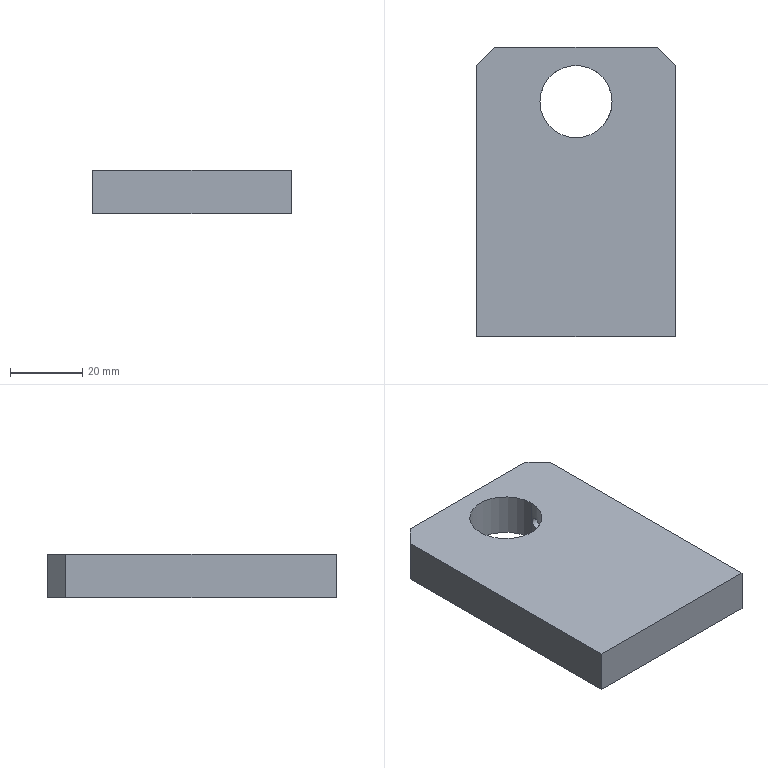Part | SolidWorks | features ICE 3, 3DProfileFeature 1, Chamfer 1, Extrusion 1, HoleWzd 1 | 1 solid | 12 faces | box 55 x 80 x 12 mm | volume 48578 mm3 | plane 8 | cylinder 4 | commonest cylinder face diameters 3.3 x2 20 x2
STEP:
#1=CARTESIAN_POINT('',(9.798,23.,7.65));
#2=VERTEX_POINT('',#1);
#3=CARTESIAN_POINT('',(9.798,23.,4.35));
#4=VERTEX_POINT('',#3);
#5=CARTESIAN_POINT('',(9.798,23.,7.65));
#6=CARTESIAN_POINT('',(9.754,22.785,7.65));
#7=CARTESIAN_POINT('',(9.702,22.57,7.607));
#8=CARTESIAN_POINT('',(9.595,22.176,7.445));
#9=CARTESIAN_POINT('',(9.539,21.994,7.325));
#10=CARTESIAN_POINT('',(9.463,21.766,7.1));
#11=CARTESIAN_POINT('',(9.439,21.696,7.016));
#12=CARTESIAN_POINT('',(9.395,21.575,6.838));
#13=CARTESIAN_POINT('',(9.376,21.523,6.744));
#14=CARTESIAN_POINT('',(9.344,21.438,6.543));
#15=CARTESIAN_POINT('',(9.332,21.405,6.437));
#16=CARTESIAN_POINT('',(9.315,21.361,6.223));
#17=CARTESIAN_POINT('',(9.31,21.35,6.114));
#18=CARTESIAN_POINT('',(9.31,21.35,5.891));
#19=CARTESIAN_POINT('',(9.314,21.361,5.782));
#20=CARTESIAN_POINT('',(9.331,21.404,5.567));
#21=CARTESIAN_POINT('',(9.344,21.437,5.461));
#22=CARTESIAN_POINT('',(9.391,21.564,5.159));
#23=CARTESIAN_POINT('',(9.437,21.688,4.977));
#24=CARTESIAN_POINT('',(9.538,21.992,4.676));
#25=CARTESIAN_POINT('',(9.595,22.174,4.556));
#26=CARTESIAN_POINT('',(9.675,22.469,4.434));
#27=CARTESIAN_POINT('',(9.702,22.573,4.403));
#28=CARTESIAN_POINT('',(9.752,22.784,4.361));
#29=CARTESIAN_POINT('',(9.776,22.891,4.35));
#30=CARTESIAN_POINT('',(9.798,23.,4.35));
#31=B_SPLINE_CURVE_WITH_KNOTS('',3,(#5,#6,#7,#8,#9,#10,#11,#12,#13,#14,#15,#16,#17,#18,#19,#20,#21,#22,#23,#24,#25,#26,#27,#28,#29,#30),.UNSPECIFIED.,.F.,.F.,(4,2,2,2,2,2,2,2,2,2,2,2,4),(0.005184,0.005841,0.006499,0.006828,0.007157,0.007485,0.007814,0.008143,0.008472,0.00913,0.009787,0.01012,0.01044),.UNSPECIFIED.);
#32=EDGE_CURVE('',#2,#4,#31,.T.);
#33=ORIENTED_EDGE('',*,*,#32,.F.);
#34=CARTESIAN_POINT('',(27.5,23.,7.65));
#35=VERTEX_POINT('',#34);
#36=CARTESIAN_POINT('',(27.5,23.,7.65));
#37=DIRECTION('',(1.,0.,0.));
#38=VECTOR('',#37,1000.);
#39=LINE('',#36,#38);
#40=EDGE_CURVE('',#2,#35,#39,.T.);
#41=ORIENTED_EDGE('',*,*,#40,.T.);
#42=CARTESIAN_POINT('',(27.5,23.,4.35));
#43=VERTEX_POINT('',#42);
#44=CARTESIAN_POINT('',(27.5,23.,6.));
#45=DIRECTION('',(1.,0.,0.));
#46=DIRECTION('',(0.,0.,-1.));
#47=AXIS2_PLACEMENT_3D('',#44,#45,#46);
#48=CIRCLE('',#47,1.65);
#49=EDGE_CURVE('',#35,#43,#48,.T.);
#50=ORIENTED_EDGE('',*,*,#49,.T.);
#51=CARTESIAN_POINT('',(27.5,23.,4.35));
#52=DIRECTION('',(1.,0.,0.));
#53=VECTOR('',#52,1000.);
#54=LINE('',#51,#53);
#55=EDGE_CURVE('',#4,#43,#54,.T.);
#56=ORIENTED_EDGE('',*,*,#55,.F.);
#57=EDGE_LOOP('',(#33,#41,#50,#56));
#58=FACE_OUTER_BOUND('',#57,.T.);
#59=CARTESIAN_POINT('',(27.5,23.,6.));
#60=DIRECTION('',(1.,0.,0.));
#61=DIRECTION('',(0.,0.,-1.));
#62=AXIS2_PLACEMENT_3D('',#59,#60,#61);
#63=CYLINDRICAL_SURFACE('',#62,1.65);
#64=ADVANCED_FACE('',(#58),#63,.F.);
#65=CARTESIAN_POINT('',(9.798,23.,4.35));
#66=CARTESIAN_POINT('',(9.82,23.107,4.35));
#67=CARTESIAN_POINT('',(9.84,23.213,4.36));
#68=CARTESIAN_POINT('',(9.875,23.422,4.401));
#69=CARTESIAN_POINT('',(9.891,23.527,4.433));
#70=CARTESIAN_POINT('',(9.919,23.726,4.514));
#71=CARTESIAN_POINT('',(9.931,23.821,4.565));
#72=CARTESIAN_POINT('',(9.95,24.001,4.684));
#73=CARTESIAN_POINT('',(9.958,24.086,4.753));
#74=CARTESIAN_POINT('',(9.978,24.316,4.982));
#75=CARTESIAN_POINT('',(9.985,24.44,5.166));
#76=CARTESIAN_POINT('',(9.993,24.606,5.565));
#77=CARTESIAN_POINT('',(9.994,24.65,5.783));
#78=CARTESIAN_POINT('',(9.994,24.65,6.108));
#79=CARTESIAN_POINT('',(9.994,24.639,6.217));
#80=CARTESIAN_POINT('',(9.992,24.597,6.43));
#81=CARTESIAN_POINT('',(9.991,24.565,6.533));
#82=CARTESIAN_POINT('',(9.987,24.482,6.734));
#83=CARTESIAN_POINT('',(9.984,24.43,6.831));
#84=CARTESIAN_POINT('',(9.976,24.309,7.01));
#85=CARTESIAN_POINT('',(9.971,24.24,7.094));
#86=CARTESIAN_POINT('',(9.958,24.085,7.248));
#87=CARTESIAN_POINT('',(9.95,24.002,7.316));
#88=CARTESIAN_POINT('',(9.931,23.822,7.435));
#89=CARTESIAN_POINT('',(9.919,23.725,7.486));
#90=CARTESIAN_POINT('',(9.891,23.526,7.568));
#91=CARTESIAN_POINT('',(9.876,23.424,7.598));
#92=CARTESIAN_POINT('',(9.84,23.214,7.64));
#93=CARTESIAN_POINT('',(9.82,23.106,7.65));
#94=CARTESIAN_POINT('',(9.798,23.,7.65));
#95=B_SPLINE_CURVE_WITH_KNOTS('',3,(#65,#66,#67,#68,#69,#70,#71,#72,#73,#74,#75,#76,#77,#78,#79,#80,#81,#82,#83,#84,#85,#86,#87,#88,#89,#90,#91,#92,#93,#94),.UNSPECIFIED.,.F.,.F.,(4,2,2,2,2,2,2,2,2,2,2,2,2,2,4),(0.,0.000324,0.0006479,0.0009719,0.001296,0.001944,0.002592,0.002916,0.00324,0.003564,0.003888,0.004212,0.004536,0.00486,0.005184),.UNSPECIFIED.);
#96=EDGE_CURVE('',#4,#2,#95,.T.);
#97=ORIENTED_EDGE('',*,*,#96,.T.);
#98=ORIENTED_EDGE('',*,*,#32,.T.);
#99=EDGE_LOOP('',(#97,#98));
#100=FACE_BOUND('',#99,.T.);
#101=CARTESIAN_POINT('',(-10.,25.,12.));
#102=VERTEX_POINT('',#101);
#103=CARTESIAN_POINT('',(10.,25.,12.));
#104=VERTEX_POINT('',#103);
#105=CARTESIAN_POINT('',(0.,25.,12.));
#106=DIRECTION('',(0.,0.,1.));
#107=DIRECTION('',(-1.,0.,0.));
#108=AXIS2_PLACEMENT_3D('',#105,#106,#107);
#109=CIRCLE('',#108,10.);
#110=EDGE_CURVE('',#102,#104,#109,.T.);
#111=ORIENTED_EDGE('',*,*,#110,.T.);
#112=CARTESIAN_POINT('',(10.,25.,0.));
#113=VERTEX_POINT('',#112);
#114=CARTESIAN_POINT('',(10.,25.,12.001));
#115=DIRECTION('',(0.,0.,-1.));
#116=VECTOR('',#115,1000.);
#117=LINE('',#114,#116);
#118=EDGE_CURVE('',#104,#113,#117,.T.);
#119=ORIENTED_EDGE('',*,*,#118,.T.);
#120=CARTESIAN_POINT('',(-10.,25.,0.));
#121=VERTEX_POINT('',#120);
#122=CARTESIAN_POINT('',(0.,25.,0.));
#123=DIRECTION('',(0.,0.,-1.));
#124=DIRECTION('',(-1.,0.,0.));
#125=AXIS2_PLACEMENT_3D('',#122,#123,#124);
#126=CIRCLE('',#125,10.);
#127=EDGE_CURVE('',#113,#121,#126,.T.);
#128=ORIENTED_EDGE('',*,*,#127,.T.);
#129=CARTESIAN_POINT('',(-10.,25.,12.001));
#130=DIRECTION('',(0.,0.,-1.));
#131=VECTOR('',#130,1000.);
#132=LINE('',#129,#131);
#133=EDGE_CURVE('',#102,#121,#132,.T.);
#134=ORIENTED_EDGE('',*,*,#133,.F.);
#135=EDGE_LOOP('',(#111,#119,#128,#134));
#136=FACE_OUTER_BOUND('',#135,.T.);
#137=CARTESIAN_POINT('',(0.,25.,12.001));
#138=DIRECTION('',(0.,0.,-1.));
#139=DIRECTION('',(-1.,0.,0.));
#140=AXIS2_PLACEMENT_3D('',#137,#138,#139);
#141=CYLINDRICAL_SURFACE('',#140,10.);
#142=ADVANCED_FACE('',(#100,#136),#141,.F.);
#143=CARTESIAN_POINT('',(27.5,-40.,0.));
#144=VERTEX_POINT('',#143);
#145=CARTESIAN_POINT('',(27.5,35.,0.));
#146=VERTEX_POINT('',#145);
#147=CARTESIAN_POINT('',(27.5,-40.,0.));
#148=DIRECTION('',(0.,1.,0.));
#149=VECTOR('',#148,1000.);
#150=LINE('',#147,#149);
#151=EDGE_CURVE('',#144,#146,#150,.T.);
#152=ORIENTED_EDGE('',*,*,#151,.T.);
#153=CARTESIAN_POINT('',(27.5,35.,12.));
#154=VERTEX_POINT('',#153);
#155=CARTESIAN_POINT('',(27.5,35.,12.));
#156=DIRECTION('',(0.,0.,1.));
#157=VECTOR('',#156,1000.);
#158=LINE('',#155,#157);
#159=EDGE_CURVE('',#146,#154,#158,.T.);
#160=ORIENTED_EDGE('',*,*,#159,.T.);
#161=CARTESIAN_POINT('',(27.5,-40.,12.));
#162=VERTEX_POINT('',#161);
#163=CARTESIAN_POINT('',(27.5,-40.,12.));
#164=DIRECTION('',(0.,1.,0.));
#165=VECTOR('',#164,1000.);
#166=LINE('',#163,#165);
#167=EDGE_CURVE('',#162,#154,#166,.T.);
#168=ORIENTED_EDGE('',*,*,#167,.F.);
#169=CARTESIAN_POINT('',(27.5,-40.,12.));
#170=DIRECTION('',(0.,0.,-1.));
#171=VECTOR('',#170,1000.);
#172=LINE('',#169,#171);
#173=EDGE_CURVE('',#162,#144,#172,.T.);
#174=ORIENTED_EDGE('',*,*,#173,.T.);
#175=EDGE_LOOP('',(#152,#160,#168,#174));
#176=FACE_OUTER_BOUND('',#175,.T.);
#177=CARTESIAN_POINT('',(27.5,23.,6.));
#178=DIRECTION('',(1.,0.,0.));
#179=DIRECTION('',(0.,0.,-1.));
#180=AXIS2_PLACEMENT_3D('',#177,#178,#179);
#181=CIRCLE('',#180,1.65);
#182=EDGE_CURVE('',#43,#35,#181,.T.);
#183=ORIENTED_EDGE('',*,*,#182,.F.);
#184=ORIENTED_EDGE('',*,*,#49,.F.);
#185=EDGE_LOOP('',(#183,#184));
#186=FACE_BOUND('',#185,.T.);
#187=CARTESIAN_POINT('',(27.5,-40.,12.));
#188=DIRECTION('',(-1.,0.,0.));
#189=DIRECTION('',(0.,0.,1.));
#190=AXIS2_PLACEMENT_3D('',#187,#188,#189);
#191=PLANE('',#190);
#192=ADVANCED_FACE('',(#176,#186),#191,.F.);
#193=CARTESIAN_POINT('',(22.5,40.,0.));
#194=VERTEX_POINT('',#193);
#195=CARTESIAN_POINT('',(-22.5,40.,0.));
#196=VERTEX_POINT('',#195);
#197=CARTESIAN_POINT('',(-27.5,40.,0.));
#198=DIRECTION('',(-1.,0.,0.));
#199=VECTOR('',#198,1000.);
#200=LINE('',#197,#199);
#201=EDGE_CURVE('',#194,#196,#200,.T.);
#202=ORIENTED_EDGE('',*,*,#201,.T.);
#203=CARTESIAN_POINT('',(-22.5,40.,12.));
#204=VERTEX_POINT('',#203);
#205=CARTESIAN_POINT('',(-22.5,40.,12.));
#206=DIRECTION('',(0.,0.,1.));
#207=VECTOR('',#206,1000.);
#208=LINE('',#205,#207);
#209=EDGE_CURVE('',#196,#204,#208,.T.);
#210=ORIENTED_EDGE('',*,*,#209,.T.);
#211=CARTESIAN_POINT('',(22.5,40.,12.));
#212=VERTEX_POINT('',#211);
#213=CARTESIAN_POINT('',(-27.5,40.,12.));
#214=DIRECTION('',(-1.,0.,0.));
#215=VECTOR('',#214,1000.);
#216=LINE('',#213,#215);
#217=EDGE_CURVE('',#212,#204,#216,.T.);
#218=ORIENTED_EDGE('',*,*,#217,.F.);
#219=CARTESIAN_POINT('',(22.5,40.,12.));
#220=DIRECTION('',(0.,0.,-1.));
#221=VECTOR('',#220,1000.);
#222=LINE('',#219,#221);
#223=EDGE_CURVE('',#212,#194,#222,.T.);
#224=ORIENTED_EDGE('',*,*,#223,.T.);
#225=EDGE_LOOP('',(#202,#210,#218,#224));
#226=FACE_OUTER_BOUND('',#225,.T.);
#227=CARTESIAN_POINT('',(-27.5,40.,12.));
#228=DIRECTION('',(0.,-1.,0.));
#229=DIRECTION('',(0.,0.,-1.));
#230=AXIS2_PLACEMENT_3D('',#227,#228,#229);
#231=PLANE('',#230);
#232=ADVANCED_FACE('',(#226),#231,.F.);
#233=CARTESIAN_POINT('',(-27.5,35.,12.));
#234=VERTEX_POINT('',#233);
#235=CARTESIAN_POINT('',(-27.5,-40.,12.));
#236=VERTEX_POINT('',#235);
#237=CARTESIAN_POINT('',(-27.5,-40.,12.));
#238=DIRECTION('',(0.,-1.,0.));
#239=VECTOR('',#238,1000.);
#240=LINE('',#237,#239);
#241=EDGE_CURVE('',#234,#236,#240,.T.);
#242=ORIENTED_EDGE('',*,*,#241,.F.);
#243=CARTESIAN_POINT('',(-27.5,35.,0.));
#244=VERTEX_POINT('',#243);
#245=CARTESIAN_POINT('',(-27.5,35.,12.));
#246=DIRECTION('',(0.,0.,-1.));
#247=VECTOR('',#246,1000.);
#248=LINE('',#245,#247);
#249=EDGE_CURVE('',#234,#244,#248,.T.);
#250=ORIENTED_EDGE('',*,*,#249,.T.);
#251=CARTESIAN_POINT('',(-27.5,-40.,0.));
#252=VERTEX_POINT('',#251);
#253=CARTESIAN_POINT('',(-27.5,-40.,0.));
#254=DIRECTION('',(0.,-1.,0.));
#255=VECTOR('',#254,1000.);
#256=LINE('',#253,#255);
#257=EDGE_CURVE('',#244,#252,#256,.T.);
#258=ORIENTED_EDGE('',*,*,#257,.T.);
#259=CARTESIAN_POINT('',(-27.5,-40.,12.));
#260=DIRECTION('',(0.,0.,-1.));
#261=VECTOR('',#260,1000.);
#262=LINE('',#259,#261);
#263=EDGE_CURVE('',#236,#252,#262,.T.);
#264=ORIENTED_EDGE('',*,*,#263,.F.);
#265=EDGE_LOOP('',(#242,#250,#258,#264));
#266=FACE_OUTER_BOUND('',#265,.T.);
#267=CARTESIAN_POINT('',(-27.5,-40.,12.));
#268=DIRECTION('',(1.,0.,0.));
#269=DIRECTION('',(0.,0.,-1.));
#270=AXIS2_PLACEMENT_3D('',#267,#268,#269);
#271=PLANE('',#270);
#272=ADVANCED_FACE('',(#266),#271,.F.);
#273=CARTESIAN_POINT('',(-27.5,-40.,0.));
#274=DIRECTION('',(1.,0.,0.));
#275=VECTOR('',#274,1000.);
#276=LINE('',#273,#275);
#277=EDGE_CURVE('',#252,#144,#276,.T.);
#278=ORIENTED_EDGE('',*,*,#277,.T.);
#279=ORIENTED_EDGE('',*,*,#173,.F.);
#280=CARTESIAN_POINT('',(-27.5,-40.,12.));
#281=DIRECTION('',(1.,0.,0.));
#282=VECTOR('',#281,1000.);
#283=LINE('',#280,#282);
#284=EDGE_CURVE('',#236,#162,#283,.T.);
#285=ORIENTED_EDGE('',*,*,#284,.F.);
#286=ORIENTED_EDGE('',*,*,#263,.T.);
#287=EDGE_LOOP('',(#278,#279,#285,#286));
#288=FACE_OUTER_BOUND('',#287,.T.);
#289=CARTESIAN_POINT('',(-27.5,-40.,12.));
#290=DIRECTION('',(0.,1.,0.));
#291=DIRECTION('',(0.,0.,1.));
#292=AXIS2_PLACEMENT_3D('',#289,#290,#291);
#293=PLANE('',#292);
#294=ADVANCED_FACE('',(#288),#293,.F.);
#295=ORIENTED_EDGE('',*,*,#110,.F.);
#296=CARTESIAN_POINT('',(0.,25.,12.));
#297=DIRECTION('',(0.,0.,1.));
#298=DIRECTION('',(-1.,0.,0.));
#299=AXIS2_PLACEMENT_3D('',#296,#297,#298);
#300=CIRCLE('',#299,10.);
#301=EDGE_CURVE('',#104,#102,#300,.T.);
#302=ORIENTED_EDGE('',*,*,#301,.F.);
#303=EDGE_LOOP('',(#295,#302));
#304=FACE_BOUND('',#303,.T.);
#305=ORIENTED_EDGE('',*,*,#217,.T.);
#306=CARTESIAN_POINT('',(-27.5,35.,12.));
#307=DIRECTION('',(-0.7071,-0.7071,0.));
#308=VECTOR('',#307,1000.);
#309=LINE('',#306,#308);
#310=EDGE_CURVE('',#204,#234,#309,.T.);
#311=ORIENTED_EDGE('',*,*,#310,.T.);
#312=ORIENTED_EDGE('',*,*,#241,.T.);
#313=ORIENTED_EDGE('',*,*,#284,.T.);
#314=ORIENTED_EDGE('',*,*,#167,.T.);
#315=CARTESIAN_POINT('',(22.5,40.,12.));
#316=DIRECTION('',(-0.7071,0.7071,0.));
#317=VECTOR('',#316,1000.);
#318=LINE('',#315,#317);
#319=EDGE_CURVE('',#154,#212,#318,.T.);
#320=ORIENTED_EDGE('',*,*,#319,.T.);
#321=EDGE_LOOP('',(#305,#311,#312,#313,#314,#320));
#322=FACE_OUTER_BOUND('',#321,.T.);
#323=CARTESIAN_POINT('',(0.,0.,12.));
#324=DIRECTION('',(0.,0.,-1.));
#325=DIRECTION('',(-1.,0.,0.));
#326=AXIS2_PLACEMENT_3D('',#323,#324,#325);
#327=PLANE('',#326);
#328=ADVANCED_FACE('',(#304,#322),#327,.F.);
#329=CARTESIAN_POINT('',(0.,25.,0.));
#330=DIRECTION('',(0.,0.,-1.));
#331=DIRECTION('',(-1.,0.,0.));
#332=AXIS2_PLACEMENT_3D('',#329,#330,#331);
#333=CIRCLE('',#332,10.);
#334=EDGE_CURVE('',#121,#113,#333,.T.);
#335=ORIENTED_EDGE('',*,*,#334,.F.);
#336=ORIENTED_EDGE('',*,*,#127,.F.);
#337=EDGE_LOOP('',(#335,#336));
#338=FACE_BOUND('',#337,.T.);
#339=ORIENTED_EDGE('',*,*,#257,.F.);
#340=CARTESIAN_POINT('',(-31.25,31.25,0.));
#341=DIRECTION('',(0.7071,0.7071,0.));
#342=VECTOR('',#341,1000.);
#343=LINE('',#340,#342);
#344=EDGE_CURVE('',#244,#196,#343,.T.);
#345=ORIENTED_EDGE('',*,*,#344,.T.);
#346=ORIENTED_EDGE('',*,*,#201,.F.);
#347=CARTESIAN_POINT('',(31.25,31.25,0.));
#348=DIRECTION('',(0.7071,-0.7071,0.));
#349=VECTOR('',#348,1000.);
#350=LINE('',#347,#349);
#351=EDGE_CURVE('',#194,#146,#350,.T.);
#352=ORIENTED_EDGE('',*,*,#351,.T.);
#353=ORIENTED_EDGE('',*,*,#151,.F.);
#354=ORIENTED_EDGE('',*,*,#277,.F.);
#355=EDGE_LOOP('',(#339,#345,#346,#352,#353,#354));
#356=FACE_OUTER_BOUND('',#355,.T.);
#357=CARTESIAN_POINT('',(0.,0.,0.));
#358=DIRECTION('',(0.,0.,-1.));
#359=DIRECTION('',(-1.,0.,0.));
#360=AXIS2_PLACEMENT_3D('',#357,#358,#359);
#361=PLANE('',#360);
#362=ADVANCED_FACE('',(#338,#356),#361,.T.);
#363=ORIENTED_EDGE('',*,*,#118,.F.);
#364=ORIENTED_EDGE('',*,*,#301,.T.);
#365=ORIENTED_EDGE('',*,*,#133,.T.);
#366=ORIENTED_EDGE('',*,*,#334,.T.);
#367=EDGE_LOOP('',(#363,#364,#365,#366));
#368=FACE_OUTER_BOUND('',#367,.T.);
#369=CARTESIAN_POINT('',(0.,25.,12.001));
#370=DIRECTION('',(0.,0.,-1.));
#371=DIRECTION('',(-1.,0.,0.));
#372=AXIS2_PLACEMENT_3D('',#369,#370,#371);
#373=CYLINDRICAL_SURFACE('',#372,10.);
#374=ADVANCED_FACE('',(#368),#373,.F.);
#375=ORIENTED_EDGE('',*,*,#310,.F.);
#376=ORIENTED_EDGE('',*,*,#209,.F.);
#377=ORIENTED_EDGE('',*,*,#344,.F.);
#378=ORIENTED_EDGE('',*,*,#249,.F.);
#379=EDGE_LOOP('',(#375,#376,#377,#378));
#380=FACE_OUTER_BOUND('',#379,.T.);
#381=CARTESIAN_POINT('',(-27.5,35.,12.));
#382=DIRECTION('',(0.7071,-0.7071,0.));
#383=DIRECTION('',(0.,0.,-1.));
#384=AXIS2_PLACEMENT_3D('',#381,#382,#383);
#385=PLANE('',#384);
#386=ADVANCED_FACE('',(#380),#385,.F.);
#387=ORIENTED_EDGE('',*,*,#319,.F.);
#388=ORIENTED_EDGE('',*,*,#159,.F.);
#389=ORIENTED_EDGE('',*,*,#351,.F.);
#390=ORIENTED_EDGE('',*,*,#223,.F.);
#391=EDGE_LOOP('',(#387,#388,#389,#390));
#392=FACE_OUTER_BOUND('',#391,.T.);
#393=CARTESIAN_POINT('',(22.5,40.,12.));
#394=DIRECTION('',(-0.7071,-0.7071,0.));
#395=DIRECTION('',(0.,0.,-1.));
#396=AXIS2_PLACEMENT_3D('',#393,#394,#395);
#397=PLANE('',#396);
#398=ADVANCED_FACE('',(#392),#397,.F.);
#399=ORIENTED_EDGE('',*,*,#40,.F.);
#400=ORIENTED_EDGE('',*,*,#96,.F.);
#401=ORIENTED_EDGE('',*,*,#55,.T.);
#402=ORIENTED_EDGE('',*,*,#182,.T.);
#403=EDGE_LOOP('',(#399,#400,#401,#402));
#404=FACE_OUTER_BOUND('',#403,.T.);
#405=CARTESIAN_POINT('',(27.5,23.,6.));
#406=DIRECTION('',(1.,0.,0.));
#407=DIRECTION('',(0.,0.,-1.));
#408=AXIS2_PLACEMENT_3D('',#405,#406,#407);
#409=CYLINDRICAL_SURFACE('',#408,1.65);
#410=ADVANCED_FACE('',(#404),#409,.F.);
#411=CLOSED_SHELL('',(#64,#142,#192,#232,#272,#294,#328,#362,#374,#386,#398,#410));
#412=MANIFOLD_SOLID_BREP('',#411);
#413=CARTESIAN_POINT('',(0.,0.,0.));
#414=DIRECTION('',(0.,0.,1.));
#415=DIRECTION('',(1.,0.,0.));
#416=AXIS2_PLACEMENT_3D('',#413,#414,#415);
#417=(LENGTH_UNIT()NAMED_UNIT(*)SI_UNIT(.MILLI.,.METRE.));
#418=UNCERTAINTY_MEASURE_WITH_UNIT(LENGTH_MEASURE(0.00001),#417,'','');
#419=(NAMED_UNIT(*)PLANE_ANGLE_UNIT()SI_UNIT($,.RADIAN.));
#420=(NAMED_UNIT(*)SI_UNIT($,.STERADIAN.)SOLID_ANGLE_UNIT());
#421=(GEOMETRIC_REPRESENTATION_CONTEXT(3)GLOBAL_UNCERTAINTY_ASSIGNED_CONTEXT((#418))GLOBAL_UNIT_ASSIGNED_CONTEXT((#417,#419,#420))REPRESENTATION_CONTEXT('',''));
#422=ADVANCED_BREP_SHAPE_REPRESENTATION('',(#412,#416),#421);